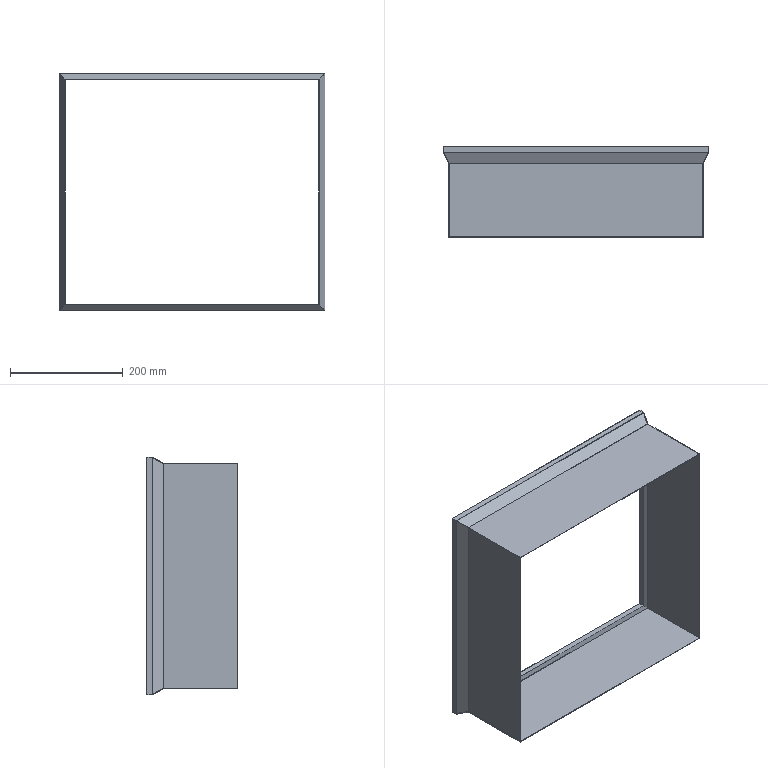Part | SolidWorks | features BaseBody 1 | 1 solid | 26 faces | box 470 x 160 x 420 mm | volume 277049 mm3 | plane 26
STEP:
#1=CARTESIAN_POINT('',(234.,85.236,-9.));
#2=VERTEX_POINT('',#1);
#3=CARTESIAN_POINT('',(-234.,85.236,-9.));
#4=VERTEX_POINT('',#3);
#5=CARTESIAN_POINT('',(0.,85.236,-9.));
#6=DIRECTION('',(-1.,0.,0.));
#7=VECTOR('',#6,1000.);
#8=LINE('',#5,#7);
#9=EDGE_CURVE('',#2,#4,#8,.T.);
#10=ORIENTED_EDGE('',*,*,#9,.F.);
#11=CARTESIAN_POINT('',(234.,95.,-9.));
#12=VERTEX_POINT('',#11);
#13=CARTESIAN_POINT('',(234.,95.,-9.));
#14=DIRECTION('',(0.,-1.,0.));
#15=VECTOR('',#14,1000.);
#16=LINE('',#13,#15);
#17=EDGE_CURVE('',#12,#2,#16,.T.);
#18=ORIENTED_EDGE('',*,*,#17,.F.);
#19=CARTESIAN_POINT('',(-234.,95.,-9.));
#20=VERTEX_POINT('',#19);
#21=CARTESIAN_POINT('',(-235.,95.,-9.));
#22=DIRECTION('',(-1.,0.,0.));
#23=VECTOR('',#22,1000.);
#24=LINE('',#21,#23);
#25=EDGE_CURVE('',#12,#20,#24,.T.);
#26=ORIENTED_EDGE('',*,*,#25,.T.);
#27=CARTESIAN_POINT('',(-234.,95.,-9.));
#28=DIRECTION('',(0.,-1.,0.));
#29=VECTOR('',#28,1000.);
#30=LINE('',#27,#29);
#31=EDGE_CURVE('',#20,#4,#30,.T.);
#32=ORIENTED_EDGE('',*,*,#31,.T.);
#33=EDGE_LOOP('',(#10,#18,#26,#32));
#34=FACE_OUTER_BOUND('',#33,.T.);
#35=CARTESIAN_POINT('',(-235.,95.,-9.));
#36=DIRECTION('',(0.,0.,1.));
#37=DIRECTION('',(1.,0.,0.));
#38=AXIS2_PLACEMENT_3D('',#35,#36,#37);
#39=PLANE('',#38);
#40=ADVANCED_FACE('',(#34),#39,.T.);
#41=CARTESIAN_POINT('',(234.,85.236,409.));
#42=VERTEX_POINT('',#41);
#43=CARTESIAN_POINT('',(234.,85.236,0.));
#44=DIRECTION('',(0.,0.,-1.));
#45=VECTOR('',#44,1000.);
#46=LINE('',#43,#45);
#47=EDGE_CURVE('',#42,#2,#46,.T.);
#48=ORIENTED_EDGE('',*,*,#47,.F.);
#49=CARTESIAN_POINT('',(234.,95.,409.));
#50=VERTEX_POINT('',#49);
#51=CARTESIAN_POINT('',(234.,95.,409.));
#52=DIRECTION('',(0.,-1.,0.));
#53=VECTOR('',#52,1000.);
#54=LINE('',#51,#53);
#55=EDGE_CURVE('',#50,#42,#54,.T.);
#56=ORIENTED_EDGE('',*,*,#55,.F.);
#57=CARTESIAN_POINT('',(234.,95.,-10.));
#58=DIRECTION('',(0.,0.,-1.));
#59=VECTOR('',#58,1000.);
#60=LINE('',#57,#59);
#61=EDGE_CURVE('',#50,#12,#60,.T.);
#62=ORIENTED_EDGE('',*,*,#61,.T.);
#63=ORIENTED_EDGE('',*,*,#17,.T.);
#64=EDGE_LOOP('',(#48,#56,#62,#63));
#65=FACE_OUTER_BOUND('',#64,.T.);
#66=CARTESIAN_POINT('',(234.,95.,-10.));
#67=DIRECTION('',(-1.,0.,0.));
#68=DIRECTION('',(0.,1.,0.));
#69=AXIS2_PLACEMENT_3D('',#66,#67,#68);
#70=PLANE('',#69);
#71=ADVANCED_FACE('',(#65),#70,.T.);
#72=CARTESIAN_POINT('',(-234.,85.236,409.));
#73=VERTEX_POINT('',#72);
#74=CARTESIAN_POINT('',(-235.,85.236,409.));
#75=DIRECTION('',(1.,0.,0.));
#76=VECTOR('',#75,1000.);
#77=LINE('',#74,#76);
#78=EDGE_CURVE('',#73,#42,#77,.T.);
#79=ORIENTED_EDGE('',*,*,#78,.F.);
#80=CARTESIAN_POINT('',(-234.,95.,409.));
#81=VERTEX_POINT('',#80);
#82=CARTESIAN_POINT('',(-234.,95.,409.));
#83=DIRECTION('',(0.,-1.,0.));
#84=VECTOR('',#83,1000.);
#85=LINE('',#82,#84);
#86=EDGE_CURVE('',#81,#73,#85,.T.);
#87=ORIENTED_EDGE('',*,*,#86,.F.);
#88=CARTESIAN_POINT('',(-235.,95.,409.));
#89=DIRECTION('',(1.,0.,0.));
#90=VECTOR('',#89,1000.);
#91=LINE('',#88,#90);
#92=EDGE_CURVE('',#81,#50,#91,.T.);
#93=ORIENTED_EDGE('',*,*,#92,.T.);
#94=ORIENTED_EDGE('',*,*,#55,.T.);
#95=EDGE_LOOP('',(#79,#87,#93,#94));
#96=FACE_OUTER_BOUND('',#95,.T.);
#97=CARTESIAN_POINT('',(-235.,95.,409.));
#98=DIRECTION('',(0.,0.,-1.));
#99=DIRECTION('',(0.,-1.,0.));
#100=AXIS2_PLACEMENT_3D('',#97,#98,#99);
#101=PLANE('',#100);
#102=ADVANCED_FACE('',(#96),#101,.T.);
#103=CARTESIAN_POINT('',(-234.,85.236,-10.));
#104=DIRECTION('',(0.,0.,1.));
#105=VECTOR('',#104,1000.);
#106=LINE('',#103,#105);
#107=EDGE_CURVE('',#4,#73,#106,.T.);
#108=ORIENTED_EDGE('',*,*,#107,.F.);
#109=ORIENTED_EDGE('',*,*,#31,.F.);
#110=CARTESIAN_POINT('',(-234.,95.,-10.));
#111=DIRECTION('',(0.,0.,1.));
#112=VECTOR('',#111,1000.);
#113=LINE('',#110,#112);
#114=EDGE_CURVE('',#20,#81,#113,.T.);
#115=ORIENTED_EDGE('',*,*,#114,.T.);
#116=ORIENTED_EDGE('',*,*,#86,.T.);
#117=EDGE_LOOP('',(#108,#109,#115,#116));
#118=FACE_OUTER_BOUND('',#117,.T.);
#119=CARTESIAN_POINT('',(-234.,95.,-10.));
#120=DIRECTION('',(1.,0.,0.));
#121=DIRECTION('',(0.,0.,-1.));
#122=AXIS2_PLACEMENT_3D('',#119,#120,#121);
#123=PLANE('',#122);
#124=ADVANCED_FACE('',(#118),#123,.T.);
#125=CARTESIAN_POINT('',(-224.,65.236,399.));
#126=VERTEX_POINT('',#125);
#127=CARTESIAN_POINT('',(-98.421,-185.921,273.421));
#128=DIRECTION('',(0.4082,-0.8165,-0.4082));
#129=VECTOR('',#128,1000.);
#130=LINE('',#127,#129);
#131=EDGE_CURVE('',#73,#126,#130,.T.);
#132=ORIENTED_EDGE('',*,*,#131,.F.);
#133=ORIENTED_EDGE('',*,*,#78,.T.);
#134=CARTESIAN_POINT('',(224.,65.236,399.));
#135=VERTEX_POINT('',#134);
#136=CARTESIAN_POINT('',(98.421,-185.921,273.421));
#137=DIRECTION('',(-0.4082,-0.8165,-0.4082));
#138=VECTOR('',#137,1000.);
#139=LINE('',#136,#138);
#140=EDGE_CURVE('',#42,#135,#139,.T.);
#141=ORIENTED_EDGE('',*,*,#140,.T.);
#142=CARTESIAN_POINT('',(0.,65.236,399.));
#143=DIRECTION('',(-1.,0.,0.));
#144=VECTOR('',#143,1000.);
#145=LINE('',#142,#144);
#146=EDGE_CURVE('',#135,#126,#145,.T.);
#147=ORIENTED_EDGE('',*,*,#146,.T.);
#148=EDGE_LOOP('',(#132,#133,#141,#147));
#149=FACE_OUTER_BOUND('',#148,.T.);
#150=CARTESIAN_POINT('',(0.,-146.553,293.106));
#151=DIRECTION('',(0.,0.4472,-0.8944));
#152=DIRECTION('',(-1.,0.,0.));
#153=AXIS2_PLACEMENT_3D('',#150,#151,#152);
#154=PLANE('',#153);
#155=ADVANCED_FACE('',(#149),#154,.T.);
#156=ORIENTED_EDGE('',*,*,#140,.F.);
#157=ORIENTED_EDGE('',*,*,#47,.T.);
#158=CARTESIAN_POINT('',(224.,65.236,1.));
#159=VERTEX_POINT('',#158);
#160=CARTESIAN_POINT('',(165.088,-52.588,59.912));
#161=DIRECTION('',(-0.4082,-0.8165,0.4082));
#162=VECTOR('',#161,1000.);
#163=LINE('',#160,#162);
#164=EDGE_CURVE('',#2,#159,#163,.T.);
#165=ORIENTED_EDGE('',*,*,#164,.T.);
#166=CARTESIAN_POINT('',(224.,65.236,0.));
#167=DIRECTION('',(0.,0.,-1.));
#168=VECTOR('',#167,1000.);
#169=LINE('',#166,#168);
#170=EDGE_CURVE('',#135,#159,#169,.T.);
#171=ORIENTED_EDGE('',*,*,#170,.F.);
#172=EDGE_LOOP('',(#156,#157,#165,#171));
#173=FACE_OUTER_BOUND('',#172,.T.);
#174=CARTESIAN_POINT('',(153.106,-76.553,0.));
#175=DIRECTION('',(0.8944,-0.4472,0.));
#176=DIRECTION('',(0.,0.,-1.));
#177=AXIS2_PLACEMENT_3D('',#174,#175,#176);
#178=PLANE('',#177);
#179=ADVANCED_FACE('',(#173),#178,.F.);
#180=CARTESIAN_POINT('',(-224.,65.236,1.));
#181=VERTEX_POINT('',#180);
#182=CARTESIAN_POINT('',(-165.088,-52.588,59.912));
#183=DIRECTION('',(0.4082,-0.8165,0.4082));
#184=VECTOR('',#183,1000.);
#185=LINE('',#182,#184);
#186=EDGE_CURVE('',#4,#181,#185,.T.);
#187=ORIENTED_EDGE('',*,*,#186,.F.);
#188=ORIENTED_EDGE('',*,*,#107,.T.);
#189=ORIENTED_EDGE('',*,*,#131,.T.);
#190=CARTESIAN_POINT('',(-224.,65.236,0.));
#191=DIRECTION('',(0.,0.,-1.));
#192=VECTOR('',#191,1000.);
#193=LINE('',#190,#192);
#194=EDGE_CURVE('',#126,#181,#193,.T.);
#195=ORIENTED_EDGE('',*,*,#194,.T.);
#196=EDGE_LOOP('',(#187,#188,#189,#195));
#197=FACE_OUTER_BOUND('',#196,.T.);
#198=CARTESIAN_POINT('',(-153.106,-76.553,0.));
#199=DIRECTION('',(0.8944,0.4472,0.));
#200=DIRECTION('',(0.,0.,-1.));
#201=AXIS2_PLACEMENT_3D('',#198,#199,#200);
#202=PLANE('',#201);
#203=ADVANCED_FACE('',(#197),#202,.T.);
#204=ORIENTED_EDGE('',*,*,#164,.F.);
#205=ORIENTED_EDGE('',*,*,#9,.T.);
#206=ORIENTED_EDGE('',*,*,#186,.T.);
#207=CARTESIAN_POINT('',(0.,65.236,1.));
#208=DIRECTION('',(-1.,0.,0.));
#209=VECTOR('',#208,1000.);
#210=LINE('',#207,#209);
#211=EDGE_CURVE('',#159,#181,#210,.T.);
#212=ORIENTED_EDGE('',*,*,#211,.F.);
#213=EDGE_LOOP('',(#204,#205,#206,#212));
#214=FACE_OUTER_BOUND('',#213,.T.);
#215=CARTESIAN_POINT('',(0.,13.447,26.894));
#216=DIRECTION('',(0.,-0.4472,-0.8944));
#217=DIRECTION('',(0.,-0.8944,0.4472));
#218=AXIS2_PLACEMENT_3D('',#215,#216,#217);
#219=PLANE('',#218);
#220=ADVANCED_FACE('',(#214),#219,.F.);
#221=CARTESIAN_POINT('',(224.,-65.,1.));
#222=VERTEX_POINT('',#221);
#223=CARTESIAN_POINT('',(224.,0.,1.));
#224=DIRECTION('',(0.,1.,0.));
#225=VECTOR('',#224,1000.);
#226=LINE('',#223,#225);
#227=EDGE_CURVE('',#222,#159,#226,.T.);
#228=ORIENTED_EDGE('',*,*,#227,.T.);
#229=ORIENTED_EDGE('',*,*,#211,.T.);
#230=CARTESIAN_POINT('',(-224.,-65.,1.));
#231=VERTEX_POINT('',#230);
#232=CARTESIAN_POINT('',(-224.,0.,1.));
#233=DIRECTION('',(0.,-1.,0.));
#234=VECTOR('',#233,1000.);
#235=LINE('',#232,#234);
#236=EDGE_CURVE('',#181,#231,#235,.T.);
#237=ORIENTED_EDGE('',*,*,#236,.T.);
#238=CARTESIAN_POINT('',(0.,-65.,1.));
#239=DIRECTION('',(1.,0.,0.));
#240=VECTOR('',#239,1000.);
#241=LINE('',#238,#240);
#242=EDGE_CURVE('',#231,#222,#241,.T.);
#243=ORIENTED_EDGE('',*,*,#242,.T.);
#244=EDGE_LOOP('',(#228,#229,#237,#243));
#245=FACE_OUTER_BOUND('',#244,.T.);
#246=CARTESIAN_POINT('',(0.,0.,1.));
#247=DIRECTION('',(0.,0.,-1.));
#248=DIRECTION('',(0.,-1.,0.));
#249=AXIS2_PLACEMENT_3D('',#246,#247,#248);
#250=PLANE('',#249);
#251=ADVANCED_FACE('',(#245),#250,.F.);
#252=CARTESIAN_POINT('',(224.,-65.,399.));
#253=VERTEX_POINT('',#252);
#254=CARTESIAN_POINT('',(224.,0.,399.));
#255=DIRECTION('',(0.,1.,0.));
#256=VECTOR('',#255,1000.);
#257=LINE('',#254,#256);
#258=EDGE_CURVE('',#253,#135,#257,.T.);
#259=ORIENTED_EDGE('',*,*,#258,.F.);
#260=CARTESIAN_POINT('',(-224.,-65.,399.));
#261=VERTEX_POINT('',#260);
#262=CARTESIAN_POINT('',(0.,-65.,399.));
#263=DIRECTION('',(1.,0.,0.));
#264=VECTOR('',#263,1000.);
#265=LINE('',#262,#264);
#266=EDGE_CURVE('',#261,#253,#265,.T.);
#267=ORIENTED_EDGE('',*,*,#266,.F.);
#268=CARTESIAN_POINT('',(-224.,0.,399.));
#269=DIRECTION('',(0.,-1.,0.));
#270=VECTOR('',#269,1000.);
#271=LINE('',#268,#270);
#272=EDGE_CURVE('',#126,#261,#271,.T.);
#273=ORIENTED_EDGE('',*,*,#272,.F.);
#274=ORIENTED_EDGE('',*,*,#146,.F.);
#275=EDGE_LOOP('',(#259,#267,#273,#274));
#276=FACE_OUTER_BOUND('',#275,.T.);
#277=CARTESIAN_POINT('',(0.,0.,399.));
#278=DIRECTION('',(0.,0.,-1.));
#279=DIRECTION('',(0.,-1.,0.));
#280=AXIS2_PLACEMENT_3D('',#277,#278,#279);
#281=PLANE('',#280);
#282=ADVANCED_FACE('',(#276),#281,.T.);
#283=ORIENTED_EDGE('',*,*,#236,.F.);
#284=ORIENTED_EDGE('',*,*,#194,.F.);
#285=ORIENTED_EDGE('',*,*,#272,.T.);
#286=CARTESIAN_POINT('',(-224.,-65.,400.));
#287=DIRECTION('',(0.,0.,-1.));
#288=VECTOR('',#287,1000.);
#289=LINE('',#286,#288);
#290=EDGE_CURVE('',#261,#231,#289,.T.);
#291=ORIENTED_EDGE('',*,*,#290,.T.);
#292=EDGE_LOOP('',(#283,#284,#285,#291));
#293=FACE_OUTER_BOUND('',#292,.T.);
#294=CARTESIAN_POINT('',(-224.,-65.,400.));
#295=DIRECTION('',(1.,0.,0.));
#296=DIRECTION('',(0.,1.,0.));
#297=AXIS2_PLACEMENT_3D('',#294,#295,#296);
#298=PLANE('',#297);
#299=ADVANCED_FACE('',(#293),#298,.T.);
#300=ORIENTED_EDGE('',*,*,#227,.F.);
#301=CARTESIAN_POINT('',(224.,-65.,400.));
#302=DIRECTION('',(0.,0.,-1.));
#303=VECTOR('',#302,1000.);
#304=LINE('',#301,#303);
#305=EDGE_CURVE('',#253,#222,#304,.T.);
#306=ORIENTED_EDGE('',*,*,#305,.F.);
#307=ORIENTED_EDGE('',*,*,#258,.T.);
#308=ORIENTED_EDGE('',*,*,#170,.T.);
#309=EDGE_LOOP('',(#300,#306,#307,#308));
#310=FACE_OUTER_BOUND('',#309,.T.);
#311=CARTESIAN_POINT('',(224.,-65.,400.));
#312=DIRECTION('',(-1.,0.,0.));
#313=DIRECTION('',(0.,0.,1.));
#314=AXIS2_PLACEMENT_3D('',#311,#312,#313);
#315=PLANE('',#314);
#316=ADVANCED_FACE('',(#310),#315,.T.);
#317=ORIENTED_EDGE('',*,*,#114,.F.);
#318=ORIENTED_EDGE('',*,*,#25,.F.);
#319=ORIENTED_EDGE('',*,*,#61,.F.);
#320=ORIENTED_EDGE('',*,*,#92,.F.);
#321=EDGE_LOOP('',(#317,#318,#319,#320));
#322=FACE_BOUND('',#321,.T.);
#323=CARTESIAN_POINT('',(-235.,95.,-10.));
#324=VERTEX_POINT('',#323);
#325=CARTESIAN_POINT('',(-235.,95.,410.));
#326=VERTEX_POINT('',#325);
#327=CARTESIAN_POINT('',(-235.,95.,-10.));
#328=DIRECTION('',(0.,0.,1.));
#329=VECTOR('',#328,1000.);
#330=LINE('',#327,#329);
#331=EDGE_CURVE('',#324,#326,#330,.T.);
#332=ORIENTED_EDGE('',*,*,#331,.T.);
#333=CARTESIAN_POINT('',(235.,95.,410.));
#334=VERTEX_POINT('',#333);
#335=CARTESIAN_POINT('',(-235.,95.,410.));
#336=DIRECTION('',(1.,0.,0.));
#337=VECTOR('',#336,1000.);
#338=LINE('',#335,#337);
#339=EDGE_CURVE('',#326,#334,#338,.T.);
#340=ORIENTED_EDGE('',*,*,#339,.T.);
#341=CARTESIAN_POINT('',(235.,95.,-10.));
#342=VERTEX_POINT('',#341);
#343=CARTESIAN_POINT('',(235.,95.,-10.));
#344=DIRECTION('',(0.,0.,-1.));
#345=VECTOR('',#344,1000.);
#346=LINE('',#343,#345);
#347=EDGE_CURVE('',#334,#342,#346,.T.);
#348=ORIENTED_EDGE('',*,*,#347,.T.);
#349=CARTESIAN_POINT('',(-235.,95.,-10.));
#350=DIRECTION('',(-1.,0.,0.));
#351=VECTOR('',#350,1000.);
#352=LINE('',#349,#351);
#353=EDGE_CURVE('',#342,#324,#352,.T.);
#354=ORIENTED_EDGE('',*,*,#353,.T.);
#355=EDGE_LOOP('',(#332,#340,#348,#354));
#356=FACE_OUTER_BOUND('',#355,.T.);
#357=CARTESIAN_POINT('',(0.,95.,0.));
#358=DIRECTION('',(0.,1.,0.));
#359=DIRECTION('',(1.,0.,0.));
#360=AXIS2_PLACEMENT_3D('',#357,#358,#359);
#361=PLANE('',#360);
#362=ADVANCED_FACE('',(#322,#356),#361,.T.);
#363=CARTESIAN_POINT('',(235.,85.,-10.));
#364=VERTEX_POINT('',#363);
#365=CARTESIAN_POINT('',(-235.,85.,-10.));
#366=VERTEX_POINT('',#365);
#367=CARTESIAN_POINT('',(-235.,85.,-10.));
#368=DIRECTION('',(-1.,0.,0.));
#369=VECTOR('',#368,1000.);
#370=LINE('',#367,#369);
#371=EDGE_CURVE('',#364,#366,#370,.T.);
#372=ORIENTED_EDGE('',*,*,#371,.T.);
#373=CARTESIAN_POINT('',(-235.,95.,-10.));
#374=DIRECTION('',(0.,-1.,0.));
#375=VECTOR('',#374,1000.);
#376=LINE('',#373,#375);
#377=EDGE_CURVE('',#324,#366,#376,.T.);
#378=ORIENTED_EDGE('',*,*,#377,.F.);
#379=ORIENTED_EDGE('',*,*,#353,.F.);
#380=CARTESIAN_POINT('',(235.,95.,-10.));
#381=DIRECTION('',(0.,-1.,0.));
#382=VECTOR('',#381,1000.);
#383=LINE('',#380,#382);
#384=EDGE_CURVE('',#342,#364,#383,.T.);
#385=ORIENTED_EDGE('',*,*,#384,.T.);
#386=EDGE_LOOP('',(#372,#378,#379,#385));
#387=FACE_OUTER_BOUND('',#386,.T.);
#388=CARTESIAN_POINT('',(-235.,95.,-10.));
#389=DIRECTION('',(0.,0.,1.));
#390=DIRECTION('',(1.,0.,0.));
#391=AXIS2_PLACEMENT_3D('',#388,#389,#390);
#392=PLANE('',#391);
#393=ADVANCED_FACE('',(#387),#392,.F.);
#394=CARTESIAN_POINT('',(235.,85.,410.));
#395=VERTEX_POINT('',#394);
#396=CARTESIAN_POINT('',(235.,85.,410.));
#397=DIRECTION('',(0.,0.,-1.));
#398=VECTOR('',#397,1000.);
#399=LINE('',#396,#398);
#400=EDGE_CURVE('',#395,#364,#399,.T.);
#401=ORIENTED_EDGE('',*,*,#400,.T.);
#402=ORIENTED_EDGE('',*,*,#384,.F.);
#403=ORIENTED_EDGE('',*,*,#347,.F.);
#404=CARTESIAN_POINT('',(235.,95.,410.));
#405=DIRECTION('',(0.,-1.,0.));
#406=VECTOR('',#405,1000.);
#407=LINE('',#404,#406);
#408=EDGE_CURVE('',#334,#395,#407,.T.);
#409=ORIENTED_EDGE('',*,*,#408,.T.);
#410=EDGE_LOOP('',(#401,#402,#403,#409));
#411=FACE_OUTER_BOUND('',#410,.T.);
#412=CARTESIAN_POINT('',(235.,95.,-10.));
#413=DIRECTION('',(-1.,0.,0.));
#414=DIRECTION('',(0.,1.,0.));
#415=AXIS2_PLACEMENT_3D('',#412,#413,#414);
#416=PLANE('',#415);
#417=ADVANCED_FACE('',(#411),#416,.F.);
#418=CARTESIAN_POINT('',(-235.,85.,410.));
#419=VERTEX_POINT('',#418);
#420=CARTESIAN_POINT('',(-235.,85.,410.));
#421=DIRECTION('',(1.,0.,0.));
#422=VECTOR('',#421,1000.);
#423=LINE('',#420,#422);
#424=EDGE_CURVE('',#419,#395,#423,.T.);
#425=ORIENTED_EDGE('',*,*,#424,.T.);
#426=ORIENTED_EDGE('',*,*,#408,.F.);
#427=ORIENTED_EDGE('',*,*,#339,.F.);
#428=CARTESIAN_POINT('',(-235.,95.,410.));
#429=DIRECTION('',(0.,-1.,0.));
#430=VECTOR('',#429,1000.);
#431=LINE('',#428,#430);
#432=EDGE_CURVE('',#326,#419,#431,.T.);
#433=ORIENTED_EDGE('',*,*,#432,.T.);
#434=EDGE_LOOP('',(#425,#426,#427,#433));
#435=FACE_OUTER_BOUND('',#434,.T.);
#436=CARTESIAN_POINT('',(-235.,95.,410.));
#437=DIRECTION('',(0.,0.,-1.));
#438=DIRECTION('',(0.,-1.,0.));
#439=AXIS2_PLACEMENT_3D('',#436,#437,#438);
#440=PLANE('',#439);
#441=ADVANCED_FACE('',(#435),#440,.F.);
#442=CARTESIAN_POINT('',(-235.,85.,410.));
#443=DIRECTION('',(0.,0.,1.));
#444=VECTOR('',#443,1000.);
#445=LINE('',#442,#444);
#446=EDGE_CURVE('',#366,#419,#445,.T.);
#447=ORIENTED_EDGE('',*,*,#446,.T.);
#448=ORIENTED_EDGE('',*,*,#432,.F.);
#449=ORIENTED_EDGE('',*,*,#331,.F.);
#450=ORIENTED_EDGE('',*,*,#377,.T.);
#451=EDGE_LOOP('',(#447,#448,#449,#450));
#452=FACE_OUTER_BOUND('',#451,.T.);
#453=CARTESIAN_POINT('',(-235.,95.,-10.));
#454=DIRECTION('',(1.,0.,0.));
#455=DIRECTION('',(0.,0.,-1.));
#456=AXIS2_PLACEMENT_3D('',#453,#454,#455);
#457=PLANE('',#456);
#458=ADVANCED_FACE('',(#452),#457,.F.);
#459=CARTESIAN_POINT('',(-225.,65.,400.));
#460=VERTEX_POINT('',#459);
#461=CARTESIAN_POINT('',(-235.,85.,410.));
#462=DIRECTION('',(0.4082,-0.8165,-0.4082));
#463=VECTOR('',#462,1000.);
#464=LINE('',#461,#463);
#465=EDGE_CURVE('',#419,#460,#464,.T.);
#466=ORIENTED_EDGE('',*,*,#465,.T.);
#467=CARTESIAN_POINT('',(225.,65.,400.));
#468=VERTEX_POINT('',#467);
#469=CARTESIAN_POINT('',(0.,65.,400.));
#470=DIRECTION('',(-1.,0.,0.));
#471=VECTOR('',#470,1000.);
#472=LINE('',#469,#471);
#473=EDGE_CURVE('',#468,#460,#472,.T.);
#474=ORIENTED_EDGE('',*,*,#473,.F.);
#475=CARTESIAN_POINT('',(235.,85.,410.));
#476=DIRECTION('',(-0.4082,-0.8165,-0.4082));
#477=VECTOR('',#476,1000.);
#478=LINE('',#475,#477);
#479=EDGE_CURVE('',#395,#468,#478,.T.);
#480=ORIENTED_EDGE('',*,*,#479,.F.);
#481=ORIENTED_EDGE('',*,*,#424,.F.);
#482=EDGE_LOOP('',(#466,#474,#480,#481));
#483=FACE_OUTER_BOUND('',#482,.T.);
#484=CARTESIAN_POINT('',(0.,-147.,294.));
#485=DIRECTION('',(0.,0.4472,-0.8944));
#486=DIRECTION('',(-1.,0.,0.));
#487=AXIS2_PLACEMENT_3D('',#484,#485,#486);
#488=PLANE('',#487);
#489=ADVANCED_FACE('',(#483),#488,.F.);
#490=ORIENTED_EDGE('',*,*,#479,.T.);
#491=CARTESIAN_POINT('',(225.,65.,0.));
#492=VERTEX_POINT('',#491);
#493=CARTESIAN_POINT('',(225.,65.,0.));
#494=DIRECTION('',(0.,0.,-1.));
#495=VECTOR('',#494,1000.);
#496=LINE('',#493,#495);
#497=EDGE_CURVE('',#468,#492,#496,.T.);
#498=ORIENTED_EDGE('',*,*,#497,.T.);
#499=CARTESIAN_POINT('',(235.,85.,-10.));
#500=DIRECTION('',(-0.4082,-0.8165,0.4082));
#501=VECTOR('',#500,1000.);
#502=LINE('',#499,#501);
#503=EDGE_CURVE('',#364,#492,#502,.T.);
#504=ORIENTED_EDGE('',*,*,#503,.F.);
#505=ORIENTED_EDGE('',*,*,#400,.F.);
#506=EDGE_LOOP('',(#490,#498,#504,#505));
#507=FACE_OUTER_BOUND('',#506,.T.);
#508=CARTESIAN_POINT('',(154.,-77.,0.));
#509=DIRECTION('',(0.8944,-0.4472,0.));
#510=DIRECTION('',(0.,0.,-1.));
#511=AXIS2_PLACEMENT_3D('',#508,#509,#510);
#512=PLANE('',#511);
#513=ADVANCED_FACE('',(#507),#512,.T.);
#514=CARTESIAN_POINT('',(-225.,65.,0.));
#515=VERTEX_POINT('',#514);
#516=CARTESIAN_POINT('',(-235.,85.,-10.));
#517=DIRECTION('',(0.4082,-0.8165,0.4082));
#518=VECTOR('',#517,1000.);
#519=LINE('',#516,#518);
#520=EDGE_CURVE('',#366,#515,#519,.T.);
#521=ORIENTED_EDGE('',*,*,#520,.T.);
#522=CARTESIAN_POINT('',(-225.,65.,400.));
#523=DIRECTION('',(0.,0.,-1.));
#524=VECTOR('',#523,1000.);
#525=LINE('',#522,#524);
#526=EDGE_CURVE('',#460,#515,#525,.T.);
#527=ORIENTED_EDGE('',*,*,#526,.F.);
#528=ORIENTED_EDGE('',*,*,#465,.F.);
#529=ORIENTED_EDGE('',*,*,#446,.F.);
#530=EDGE_LOOP('',(#521,#527,#528,#529));
#531=FACE_OUTER_BOUND('',#530,.T.);
#532=CARTESIAN_POINT('',(-154.,-77.,0.));
#533=DIRECTION('',(0.8944,0.4472,0.));
#534=DIRECTION('',(0.,0.,-1.));
#535=AXIS2_PLACEMENT_3D('',#532,#533,#534);
#536=PLANE('',#535);
#537=ADVANCED_FACE('',(#531),#536,.F.);
#538=ORIENTED_EDGE('',*,*,#503,.T.);
#539=CARTESIAN_POINT('',(0.,65.,0.));
#540=DIRECTION('',(-1.,0.,0.));
#541=VECTOR('',#540,1000.);
#542=LINE('',#539,#541);
#543=EDGE_CURVE('',#492,#515,#542,.T.);
#544=ORIENTED_EDGE('',*,*,#543,.T.);
#545=ORIENTED_EDGE('',*,*,#520,.F.);
#546=ORIENTED_EDGE('',*,*,#371,.F.);
#547=EDGE_LOOP('',(#538,#544,#545,#546));
#548=FACE_OUTER_BOUND('',#547,.T.);
#549=CARTESIAN_POINT('',(0.,13.,26.));
#550=DIRECTION('',(0.,-0.4472,-0.8944));
#551=DIRECTION('',(0.,-0.8944,0.4472));
#552=AXIS2_PLACEMENT_3D('',#549,#550,#551);
#553=PLANE('',#552);
#554=ADVANCED_FACE('',(#548),#553,.T.);
#555=CARTESIAN_POINT('',(225.,-65.,0.));
#556=VERTEX_POINT('',#555);
#557=CARTESIAN_POINT('',(225.,-65.,0.));
#558=DIRECTION('',(0.,1.,0.));
#559=VECTOR('',#558,1000.);
#560=LINE('',#557,#559);
#561=EDGE_CURVE('',#556,#492,#560,.T.);
#562=ORIENTED_EDGE('',*,*,#561,.F.);
#563=CARTESIAN_POINT('',(-225.,-65.,0.));
#564=VERTEX_POINT('',#563);
#565=CARTESIAN_POINT('',(-225.,-65.,0.));
#566=DIRECTION('',(1.,0.,0.));
#567=VECTOR('',#566,1000.);
#568=LINE('',#565,#567);
#569=EDGE_CURVE('',#564,#556,#568,.T.);
#570=ORIENTED_EDGE('',*,*,#569,.F.);
#571=CARTESIAN_POINT('',(-225.,-65.,0.));
#572=DIRECTION('',(0.,-1.,0.));
#573=VECTOR('',#572,1000.);
#574=LINE('',#571,#573);
#575=EDGE_CURVE('',#515,#564,#574,.T.);
#576=ORIENTED_EDGE('',*,*,#575,.F.);
#577=ORIENTED_EDGE('',*,*,#543,.F.);
#578=EDGE_LOOP('',(#562,#570,#576,#577));
#579=FACE_OUTER_BOUND('',#578,.T.);
#580=CARTESIAN_POINT('',(0.,0.,0.));
#581=DIRECTION('',(0.,0.,-1.));
#582=DIRECTION('',(0.,-1.,0.));
#583=AXIS2_PLACEMENT_3D('',#580,#581,#582);
#584=PLANE('',#583);
#585=ADVANCED_FACE('',(#579),#584,.T.);
#586=CARTESIAN_POINT('',(225.,-65.,400.));
#587=VERTEX_POINT('',#586);
#588=CARTESIAN_POINT('',(225.,-65.,400.));
#589=DIRECTION('',(0.,1.,0.));
#590=VECTOR('',#589,1000.);
#591=LINE('',#588,#590);
#592=EDGE_CURVE('',#587,#468,#591,.T.);
#593=ORIENTED_EDGE('',*,*,#592,.T.);
#594=ORIENTED_EDGE('',*,*,#473,.T.);
#595=CARTESIAN_POINT('',(-225.,-65.,400.));
#596=VERTEX_POINT('',#595);
#597=CARTESIAN_POINT('',(-225.,-65.,400.));
#598=DIRECTION('',(0.,-1.,0.));
#599=VECTOR('',#598,1000.);
#600=LINE('',#597,#599);
#601=EDGE_CURVE('',#460,#596,#600,.T.);
#602=ORIENTED_EDGE('',*,*,#601,.T.);
#603=CARTESIAN_POINT('',(-225.,-65.,400.));
#604=DIRECTION('',(1.,0.,0.));
#605=VECTOR('',#604,1000.);
#606=LINE('',#603,#605);
#607=EDGE_CURVE('',#596,#587,#606,.T.);
#608=ORIENTED_EDGE('',*,*,#607,.T.);
#609=EDGE_LOOP('',(#593,#594,#602,#608));
#610=FACE_OUTER_BOUND('',#609,.T.);
#611=CARTESIAN_POINT('',(0.,0.,400.));
#612=DIRECTION('',(0.,0.,-1.));
#613=DIRECTION('',(0.,-1.,0.));
#614=AXIS2_PLACEMENT_3D('',#611,#612,#613);
#615=PLANE('',#614);
#616=ADVANCED_FACE('',(#610),#615,.F.);
#617=ORIENTED_EDGE('',*,*,#575,.T.);
#618=CARTESIAN_POINT('',(-225.,-65.,400.));
#619=DIRECTION('',(0.,0.,-1.));
#620=VECTOR('',#619,1000.);
#621=LINE('',#618,#620);
#622=EDGE_CURVE('',#596,#564,#621,.T.);
#623=ORIENTED_EDGE('',*,*,#622,.F.);
#624=ORIENTED_EDGE('',*,*,#601,.F.);
#625=ORIENTED_EDGE('',*,*,#526,.T.);
#626=EDGE_LOOP('',(#617,#623,#624,#625));
#627=FACE_OUTER_BOUND('',#626,.T.);
#628=CARTESIAN_POINT('',(-225.,-65.,400.));
#629=DIRECTION('',(1.,0.,0.));
#630=DIRECTION('',(0.,1.,0.));
#631=AXIS2_PLACEMENT_3D('',#628,#629,#630);
#632=PLANE('',#631);
#633=ADVANCED_FACE('',(#627),#632,.F.);
#634=ORIENTED_EDGE('',*,*,#561,.T.);
#635=ORIENTED_EDGE('',*,*,#497,.F.);
#636=ORIENTED_EDGE('',*,*,#592,.F.);
#637=CARTESIAN_POINT('',(225.,-65.,400.));
#638=DIRECTION('',(0.,0.,-1.));
#639=VECTOR('',#638,1000.);
#640=LINE('',#637,#639);
#641=EDGE_CURVE('',#587,#556,#640,.T.);
#642=ORIENTED_EDGE('',*,*,#641,.T.);
#643=EDGE_LOOP('',(#634,#635,#636,#642));
#644=FACE_OUTER_BOUND('',#643,.T.);
#645=CARTESIAN_POINT('',(225.,-65.,400.));
#646=DIRECTION('',(-1.,0.,0.));
#647=DIRECTION('',(0.,0.,1.));
#648=AXIS2_PLACEMENT_3D('',#645,#646,#647);
#649=PLANE('',#648);
#650=ADVANCED_FACE('',(#644),#649,.F.);
#651=ORIENTED_EDGE('',*,*,#242,.F.);
#652=ORIENTED_EDGE('',*,*,#290,.F.);
#653=ORIENTED_EDGE('',*,*,#266,.T.);
#654=ORIENTED_EDGE('',*,*,#305,.T.);
#655=EDGE_LOOP('',(#651,#652,#653,#654));
#656=FACE_BOUND('',#655,.T.);
#657=ORIENTED_EDGE('',*,*,#569,.T.);
#658=ORIENTED_EDGE('',*,*,#641,.F.);
#659=ORIENTED_EDGE('',*,*,#607,.F.);
#660=ORIENTED_EDGE('',*,*,#622,.T.);
#661=EDGE_LOOP('',(#657,#658,#659,#660));
#662=FACE_OUTER_BOUND('',#661,.T.);
#663=CARTESIAN_POINT('',(-225.,-65.,400.));
#664=DIRECTION('',(0.,1.,0.));
#665=DIRECTION('',(1.,0.,0.));
#666=AXIS2_PLACEMENT_3D('',#663,#664,#665);
#667=PLANE('',#666);
#668=ADVANCED_FACE('',(#656,#662),#667,.F.);
#669=CLOSED_SHELL('',(#40,#71,#102,#124,#155,#179,#203,#220,#251,#282,#299,#316,#362,#393,#417,#441,#458,#489,#513,#537,#554,#585,#616,#633,#650,#668));
#670=MANIFOLD_SOLID_BREP('',#669);
#671=CARTESIAN_POINT('',(0.,0.,0.));
#672=DIRECTION('',(0.,0.,1.));
#673=DIRECTION('',(1.,0.,0.));
#674=AXIS2_PLACEMENT_3D('',#671,#672,#673);
#675=(LENGTH_UNIT()NAMED_UNIT(*)SI_UNIT(.MILLI.,.METRE.));
#676=UNCERTAINTY_MEASURE_WITH_UNIT(LENGTH_MEASURE(0.00001),#675,'','');
#677=(NAMED_UNIT(*)PLANE_ANGLE_UNIT()SI_UNIT($,.RADIAN.));
#678=(NAMED_UNIT(*)SI_UNIT($,.STERADIAN.)SOLID_ANGLE_UNIT());
#679=(GEOMETRIC_REPRESENTATION_CONTEXT(3)GLOBAL_UNCERTAINTY_ASSIGNED_CONTEXT((#676))GLOBAL_UNIT_ASSIGNED_CONTEXT((#675,#677,#678))REPRESENTATION_CONTEXT('',''));
#680=ADVANCED_BREP_SHAPE_REPRESENTATION('',(#670,#674),#679);